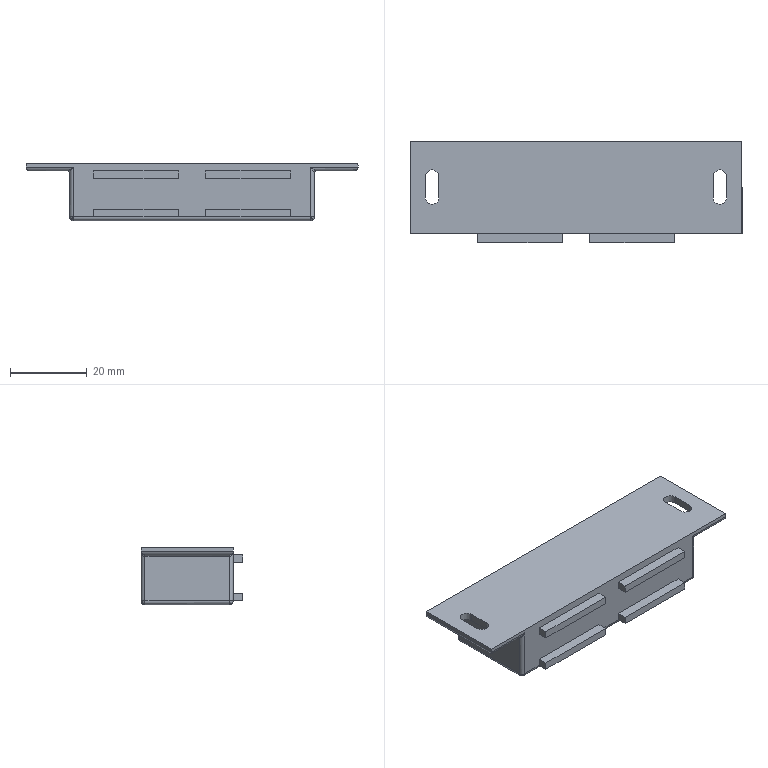Part | SolidWorks | features BaseBody 1 | 1 solid | 66 faces | box 86.5 x 26.5 x 15 mm | volume 24316 mm3 | plane 34 | cylinder 20 | spline 12 | commonest cylinder face diameters 2 x14 3.5 x4 1 x2